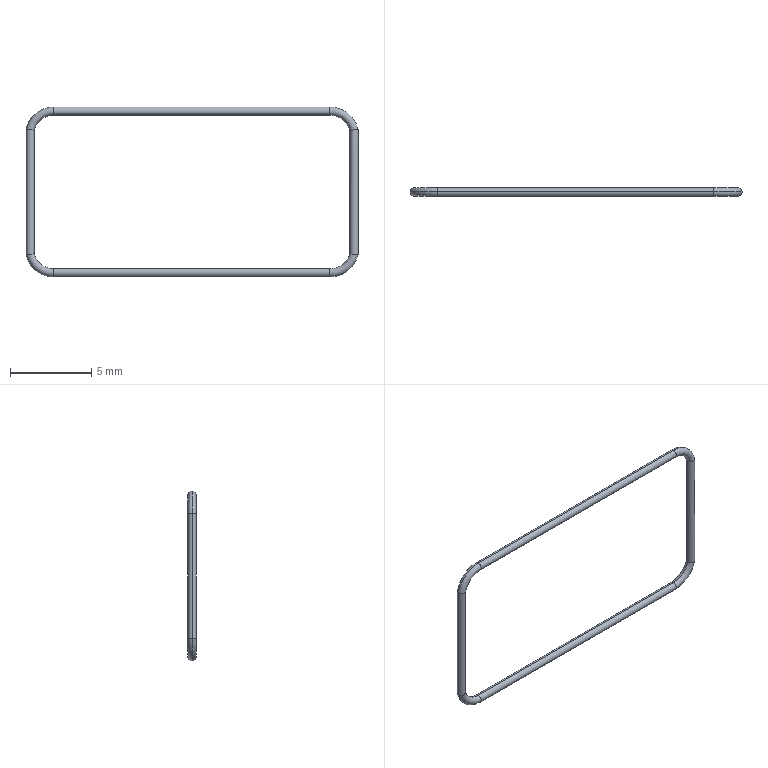Part | STEP file | XINAQUAN11_1_1_1 | 1 solid | 18 faces | box 20.47 x 0.5 x 10.48 mm | volume 11.282 mm3 | torus 8 | cylinder 8 | plane 2 | commonest cylinder face diameters 0.5 x8
STEP:
#1=CARTESIAN_POINT('',(0.,0.,0.));
#2=DIRECTION('',(0.,0.,1.));
#3=DIRECTION('',(1.,0.,0.));
#4=AXIS2_PLACEMENT_3D('',#1,#2,#3);
#5=CARTESIAN_POINT('',(8.51,0.,5.24));
#6=VERTEX_POINT('',#5);
#7=CARTESIAN_POINT('',(8.51,0.,4.74));
#8=VERTEX_POINT('',#7);
#9=CARTESIAN_POINT('',(8.51,0.,4.99));
#10=DIRECTION('',(-1.,0.,0.));
#11=DIRECTION('',(0.,0.,1.));
#12=AXIS2_PLACEMENT_3D('',#9,#10,#11);
#13=CIRCLE('',#12,0.25);
#14=EDGE_CURVE('',#6,#8,#13,.T.);
#15=ORIENTED_EDGE('',*,*,#14,.T.);
#16=CARTESIAN_POINT('',(9.758,0.,3.775));
#17=VERTEX_POINT('',#16);
#18=CARTESIAN_POINT('',(8.51,0.,3.45));
#19=DIRECTION('',(0.,1.,0.));
#20=DIRECTION('',(0.,0.,1.));
#21=AXIS2_PLACEMENT_3D('',#18,#19,#20);
#22=CIRCLE('',#21,1.29);
#23=EDGE_CURVE('',#8,#17,#22,.T.);
#24=ORIENTED_EDGE('',*,*,#23,.T.);
#25=CARTESIAN_POINT('',(10.242,0.,3.901));
#26=VERTEX_POINT('',#25);
#27=CARTESIAN_POINT('',(10.,0.,3.838));
#28=DIRECTION('',(-0.2522,0.,0.9677));
#29=DIRECTION('',(0.9677,0.,0.2522));
#30=AXIS2_PLACEMENT_3D('',#27,#28,#29);
#31=CIRCLE('',#30,0.25);
#32=EDGE_CURVE('',#26,#17,#31,.T.);
#33=ORIENTED_EDGE('',*,*,#32,.F.);
#34=CARTESIAN_POINT('',(8.51,0.,3.45));
#35=DIRECTION('',(0.,1.,0.));
#36=DIRECTION('',(0.,0.,1.));
#37=AXIS2_PLACEMENT_3D('',#34,#35,#36);
#38=CIRCLE('',#37,1.79);
#39=EDGE_CURVE('',#6,#26,#38,.T.);
#40=ORIENTED_EDGE('',*,*,#39,.F.);
#41=EDGE_LOOP('',(#15,#24,#33,#40));
#42=FACE_OUTER_BOUND('',#41,.F.);
#43=CARTESIAN_POINT('',(8.51,0.,3.45));
#44=DIRECTION('',(0.,1.,0.));
#45=DIRECTION('',(0.,0.,-1.));
#46=AXIS2_PLACEMENT_3D('',#43,#44,#45);
#47=TOROIDAL_SURFACE('',#46,1.54,0.25);
#48=ADVANCED_FACE('',(#42),#47,.T.);
#49=CARTESIAN_POINT('',(-8.51,0.,4.74));
#50=VERTEX_POINT('',#49);
#51=CARTESIAN_POINT('',(-8.51,0.,5.24));
#52=VERTEX_POINT('',#51);
#53=CARTESIAN_POINT('',(-8.51,0.,4.99));
#54=DIRECTION('',(1.,0.,0.));
#55=DIRECTION('',(0.,0.,-1.));
#56=AXIS2_PLACEMENT_3D('',#53,#54,#55);
#57=CIRCLE('',#56,0.25);
#58=EDGE_CURVE('',#50,#52,#57,.T.);
#59=ORIENTED_EDGE('',*,*,#58,.F.);
#60=CARTESIAN_POINT('',(-8.51,0.,4.74));
#61=DIRECTION('',(1.,0.,0.));
#62=VECTOR('',#61,17.02);
#63=LINE('',#60,#62);
#64=EDGE_CURVE('',#50,#8,#63,.T.);
#65=ORIENTED_EDGE('',*,*,#64,.T.);
#66=ORIENTED_EDGE('',*,*,#14,.F.);
#67=CARTESIAN_POINT('',(-8.51,0.,5.24));
#68=DIRECTION('',(1.,0.,0.));
#69=VECTOR('',#68,17.02);
#70=LINE('',#67,#69);
#71=EDGE_CURVE('',#52,#6,#70,.T.);
#72=ORIENTED_EDGE('',*,*,#71,.F.);
#73=EDGE_LOOP('',(#59,#65,#66,#72));
#74=FACE_OUTER_BOUND('',#73,.F.);
#75=CARTESIAN_POINT('',(-8.51,0.,4.99));
#76=DIRECTION('',(1.,0.,0.));
#77=DIRECTION('',(0.,0.,1.));
#78=AXIS2_PLACEMENT_3D('',#75,#76,#77);
#79=CYLINDRICAL_SURFACE('',#78,0.25);
#80=ADVANCED_FACE('',(#74),#79,.T.);
#81=CARTESIAN_POINT('',(-9.72,0.,3.805));
#82=VERTEX_POINT('',#81);
#83=CARTESIAN_POINT('',(-9.97,0.25,3.835));
#84=VERTEX_POINT('',#83);
#85=CARTESIAN_POINT('',(-9.72,0.02605,3.805));
#86=CARTESIAN_POINT('',(-9.728,0.0782,3.806));
#87=CARTESIAN_POINT('',(-9.764,0.1492,3.81));
#88=CARTESIAN_POINT('',(-9.82,0.2053,3.817));
#89=CARTESIAN_POINT('',(-9.891,0.2416,3.826));
#90=CARTESIAN_POINT('',(-9.943,0.25,3.832));
#91=B_SPLINE_CURVE_WITH_KNOTS('',3,(#81,#85,#86,#87,#88,#89,#90,#83),.UNSPECIFIED.,.F.,.F.,(4,1,1,1,1,4),(0.,0.2,0.4,0.6,0.8,1.),.UNSPECIFIED.);
#92=EDGE_CURVE('',#82,#84,#91,.T.);
#93=ORIENTED_EDGE('',*,*,#92,.F.);
#94=CARTESIAN_POINT('',(-8.51,0.,3.49));
#95=DIRECTION('',(0.,1.,0.));
#96=DIRECTION('',(-0.9678,0.,0.2516));
#97=AXIS2_PLACEMENT_3D('',#94,#95,#96);
#98=CIRCLE('',#97,1.25);
#99=EDGE_CURVE('',#82,#50,#98,.T.);
#100=ORIENTED_EDGE('',*,*,#99,.T.);
#101=ORIENTED_EDGE('',*,*,#58,.T.);
#102=CARTESIAN_POINT('',(-10.213,0.,3.893));
#103=VERTEX_POINT('',#102);
#104=CARTESIAN_POINT('',(-8.51,0.,3.49));
#105=DIRECTION('',(0.,1.,0.));
#106=DIRECTION('',(-0.9732,0.,0.23));
#107=AXIS2_PLACEMENT_3D('',#104,#105,#106);
#108=CIRCLE('',#107,1.75);
#109=EDGE_CURVE('',#103,#52,#108,.T.);
#110=ORIENTED_EDGE('',*,*,#109,.F.);
#111=CARTESIAN_POINT('',(-10.22,0.,3.863));
#112=VERTEX_POINT('',#111);
#113=CARTESIAN_POINT('',(-8.51,0.,3.49));
#114=DIRECTION('',(0.,1.,0.));
#115=DIRECTION('',(-0.977,0.,0.2131));
#116=AXIS2_PLACEMENT_3D('',#113,#114,#115);
#117=CIRCLE('',#116,1.75);
#118=EDGE_CURVE('',#112,#103,#117,.T.);
#119=ORIENTED_EDGE('',*,*,#118,.F.);
#120=CARTESIAN_POINT('',(-9.97,0.25,3.835));
#121=CARTESIAN_POINT('',(-9.996,0.25,3.838));
#122=CARTESIAN_POINT('',(-10.049,0.2416,3.844));
#123=CARTESIAN_POINT('',(-10.119,0.2055,3.852));
#124=CARTESIAN_POINT('',(-10.176,0.1491,3.858));
#125=CARTESIAN_POINT('',(-10.212,0.07816,3.862));
#126=CARTESIAN_POINT('',(-10.22,0.02602,3.863));
#127=CARTESIAN_POINT('',(-10.22,0.,3.863));
#128=B_SPLINE_CURVE_WITH_KNOTS('',3,(#120,#121,#122,#123,#124,#125,#126,#127),.UNSPECIFIED.,.F.,.F.,(4,1,1,1,1,4),(0.,0.2,0.4,0.6,0.8,1.),.UNSPECIFIED.);
#129=EDGE_CURVE('',#84,#112,#128,.T.);
#130=ORIENTED_EDGE('',*,*,#129,.F.);
#131=EDGE_LOOP('',(#93,#100,#101,#110,#119,#130));
#132=FACE_OUTER_BOUND('',#131,.F.);
#133=CARTESIAN_POINT('',(-8.51,0.,3.49));
#134=DIRECTION('',(0.,1.,0.));
#135=DIRECTION('',(0.9732,0.,-0.23));
#136=AXIS2_PLACEMENT_3D('',#133,#134,#135);
#137=TOROIDAL_SURFACE('',#136,1.5,0.25);
#138=ADVANCED_FACE('',(#132),#137,.T.);
#139=CARTESIAN_POINT('',(-9.72,0.,-3.805));
#140=VERTEX_POINT('',#139);
#141=CARTESIAN_POINT('',(-9.97,0.25,-3.835));
#142=VERTEX_POINT('',#141);
#143=CARTESIAN_POINT('',(-9.72,0.02606,-3.805));
#144=CARTESIAN_POINT('',(-9.728,0.07824,-3.806));
#145=CARTESIAN_POINT('',(-9.764,0.1492,-3.81));
#146=CARTESIAN_POINT('',(-9.82,0.2054,-3.817));
#147=CARTESIAN_POINT('',(-9.891,0.2416,-3.826));
#148=CARTESIAN_POINT('',(-9.943,0.25,-3.832));
#149=B_SPLINE_CURVE_WITH_KNOTS('',3,(#139,#143,#144,#145,#146,#147,#148,#141),.UNSPECIFIED.,.F.,.F.,(4,1,1,1,1,4),(0.,0.2,0.4,0.6,0.8,1.),.UNSPECIFIED.);
#150=EDGE_CURVE('',#140,#142,#149,.T.);
#151=ORIENTED_EDGE('',*,*,#150,.F.);
#152=CARTESIAN_POINT('',(-9.72,0.,-3.805));
#153=DIRECTION('',(0.,0.,1.));
#154=VECTOR('',#153,7.609);
#155=LINE('',#152,#154);
#156=EDGE_CURVE('',#140,#82,#155,.T.);
#157=ORIENTED_EDGE('',*,*,#156,.T.);
#158=ORIENTED_EDGE('',*,*,#92,.T.);
#159=ORIENTED_EDGE('',*,*,#129,.T.);
#160=CARTESIAN_POINT('',(-10.22,0.,-3.863));
#161=VERTEX_POINT('',#160);
#162=CARTESIAN_POINT('',(-10.22,0.,-3.863));
#163=DIRECTION('',(0.,0.,1.));
#164=VECTOR('',#163,7.726);
#165=LINE('',#162,#164);
#166=EDGE_CURVE('',#161,#112,#165,.T.);
#167=ORIENTED_EDGE('',*,*,#166,.F.);
#168=CARTESIAN_POINT('',(-9.97,0.25,-3.835));
#169=CARTESIAN_POINT('',(-9.996,0.25,-3.838));
#170=CARTESIAN_POINT('',(-10.049,0.2416,-3.844));
#171=CARTESIAN_POINT('',(-10.119,0.2055,-3.852));
#172=CARTESIAN_POINT('',(-10.176,0.1491,-3.858));
#173=CARTESIAN_POINT('',(-10.212,0.07808,-3.862));
#174=CARTESIAN_POINT('',(-10.22,0.02599,-3.863));
#175=CARTESIAN_POINT('',(-10.22,0.,-3.863));
#176=B_SPLINE_CURVE_WITH_KNOTS('',3,(#168,#169,#170,#171,#172,#173,#174,#175),.UNSPECIFIED.,.F.,.F.,(4,1,1,1,1,4),(0.,0.2,0.4,0.6,0.8,1.),.UNSPECIFIED.);
#177=EDGE_CURVE('',#142,#161,#176,.T.);
#178=ORIENTED_EDGE('',*,*,#177,.F.);
#179=EDGE_LOOP('',(#151,#157,#158,#159,#167,#178));
#180=FACE_OUTER_BOUND('',#179,.F.);
#181=CARTESIAN_POINT('',(-9.97,0.,-3.835));
#182=DIRECTION('',(0.,0.,1.));
#183=DIRECTION('',(-1.,0.,0.));
#184=AXIS2_PLACEMENT_3D('',#181,#182,#183);
#185=CYLINDRICAL_SURFACE('',#184,0.25);
#186=ADVANCED_FACE('',(#180),#185,.T.);
#187=CARTESIAN_POINT('',(-8.51,0.,-5.24));
#188=VERTEX_POINT('',#187);
#189=CARTESIAN_POINT('',(-8.51,0.,-4.74));
#190=VERTEX_POINT('',#189);
#191=CARTESIAN_POINT('',(-8.51,0.,-4.99));
#192=DIRECTION('',(1.,0.,0.));
#193=DIRECTION('',(0.,0.,-1.));
#194=AXIS2_PLACEMENT_3D('',#191,#192,#193);
#195=CIRCLE('',#194,0.25);
#196=EDGE_CURVE('',#188,#190,#195,.T.);
#197=ORIENTED_EDGE('',*,*,#196,.T.);
#198=CARTESIAN_POINT('',(-8.51,0.,-3.49));
#199=DIRECTION('',(0.,1.,0.));
#200=DIRECTION('',(0.,0.,-1.));
#201=AXIS2_PLACEMENT_3D('',#198,#199,#200);
#202=CIRCLE('',#201,1.25);
#203=EDGE_CURVE('',#190,#140,#202,.T.);
#204=ORIENTED_EDGE('',*,*,#203,.T.);
#205=ORIENTED_EDGE('',*,*,#150,.T.);
#206=ORIENTED_EDGE('',*,*,#177,.T.);
#207=CARTESIAN_POINT('',(-8.51,0.,-3.49));
#208=DIRECTION('',(0.,1.,0.));
#209=DIRECTION('',(0.,0.,-1.));
#210=AXIS2_PLACEMENT_3D('',#207,#208,#209);
#211=CIRCLE('',#210,1.75);
#212=EDGE_CURVE('',#188,#161,#211,.T.);
#213=ORIENTED_EDGE('',*,*,#212,.F.);
#214=EDGE_LOOP('',(#197,#204,#205,#206,#213));
#215=FACE_OUTER_BOUND('',#214,.F.);
#216=CARTESIAN_POINT('',(-8.51,0.,-3.49));
#217=DIRECTION('',(0.,1.,0.));
#218=DIRECTION('',(0.,0.,1.));
#219=AXIS2_PLACEMENT_3D('',#216,#217,#218);
#220=TOROIDAL_SURFACE('',#219,1.5,0.25);
#221=ADVANCED_FACE('',(#215),#220,.T.);
#222=CARTESIAN_POINT('',(8.51,0.,-4.74));
#223=VERTEX_POINT('',#222);
#224=CARTESIAN_POINT('',(8.51,0.,-5.24));
#225=VERTEX_POINT('',#224);
#226=CARTESIAN_POINT('',(8.51,0.,-4.99));
#227=DIRECTION('',(-1.,0.,0.));
#228=DIRECTION('',(0.,0.,1.));
#229=AXIS2_PLACEMENT_3D('',#226,#227,#228);
#230=CIRCLE('',#229,0.25);
#231=EDGE_CURVE('',#223,#225,#230,.T.);
#232=ORIENTED_EDGE('',*,*,#231,.F.);
#233=CARTESIAN_POINT('',(8.51,0.,-4.74));
#234=DIRECTION('',(-1.,0.,0.));
#235=VECTOR('',#234,17.02);
#236=LINE('',#233,#235);
#237=EDGE_CURVE('',#223,#190,#236,.T.);
#238=ORIENTED_EDGE('',*,*,#237,.T.);
#239=ORIENTED_EDGE('',*,*,#196,.F.);
#240=CARTESIAN_POINT('',(8.51,0.,-5.24));
#241=DIRECTION('',(-1.,0.,0.));
#242=VECTOR('',#241,17.02);
#243=LINE('',#240,#242);
#244=EDGE_CURVE('',#225,#188,#243,.T.);
#245=ORIENTED_EDGE('',*,*,#244,.F.);
#246=EDGE_LOOP('',(#232,#238,#239,#245));
#247=FACE_OUTER_BOUND('',#246,.F.);
#248=CARTESIAN_POINT('',(8.51,0.,-4.99));
#249=DIRECTION('',(-1.,0.,0.));
#250=DIRECTION('',(0.,0.,-1.));
#251=AXIS2_PLACEMENT_3D('',#248,#249,#250);
#252=CYLINDRICAL_SURFACE('',#251,0.25);
#253=ADVANCED_FACE('',(#247),#252,.T.);
#254=CARTESIAN_POINT('',(9.75,0.,-3.805));
#255=VERTEX_POINT('',#254);
#256=CARTESIAN_POINT('',(10.,0.25,-3.838));
#257=VERTEX_POINT('',#256);
#258=CARTESIAN_POINT('',(9.75,0.02603,-3.805));
#259=CARTESIAN_POINT('',(9.758,0.07815,-3.806));
#260=CARTESIAN_POINT('',(9.794,0.1491,-3.811));
#261=CARTESIAN_POINT('',(9.85,0.2053,-3.819));
#262=CARTESIAN_POINT('',(9.921,0.2415,-3.828));
#263=CARTESIAN_POINT('',(9.974,0.25,-3.835));
#264=B_SPLINE_CURVE_WITH_KNOTS('',3,(#254,#258,#259,#260,#261,#262,#263,#256),.UNSPECIFIED.,.F.,.F.,(4,1,1,1,1,4),(0.,0.2,0.4,0.6,0.8,1.),.UNSPECIFIED.);
#265=EDGE_CURVE('',#255,#257,#264,.T.);
#266=ORIENTED_EDGE('',*,*,#265,.F.);
#267=CARTESIAN_POINT('',(8.51,0.,-3.45));
#268=DIRECTION('',(0.,1.,0.));
#269=DIRECTION('',(0.9614,0.,-0.2751));
#270=AXIS2_PLACEMENT_3D('',#267,#268,#269);
#271=CIRCLE('',#270,1.29);
#272=EDGE_CURVE('',#255,#223,#271,.T.);
#273=ORIENTED_EDGE('',*,*,#272,.T.);
#274=ORIENTED_EDGE('',*,*,#231,.T.);
#275=CARTESIAN_POINT('',(10.242,0.,-3.901));
#276=VERTEX_POINT('',#275);
#277=CARTESIAN_POINT('',(8.51,0.,-3.45));
#278=DIRECTION('',(0.,1.,0.));
#279=DIRECTION('',(0.9677,0.,-0.2522));
#280=AXIS2_PLACEMENT_3D('',#277,#278,#279);
#281=CIRCLE('',#280,1.79);
#282=EDGE_CURVE('',#276,#225,#281,.T.);
#283=ORIENTED_EDGE('',*,*,#282,.F.);
#284=CARTESIAN_POINT('',(10.25,0.,-3.869));
#285=VERTEX_POINT('',#284);
#286=CARTESIAN_POINT('',(8.51,0.,-3.45));
#287=DIRECTION('',(0.,1.,0.));
#288=DIRECTION('',(0.9722,0.,-0.2342));
#289=AXIS2_PLACEMENT_3D('',#286,#287,#288);
#290=CIRCLE('',#289,1.79);
#291=EDGE_CURVE('',#285,#276,#290,.T.);
#292=ORIENTED_EDGE('',*,*,#291,.F.);
#293=CARTESIAN_POINT('',(10.,0.25,-3.838));
#294=CARTESIAN_POINT('',(10.027,0.25,-3.842));
#295=CARTESIAN_POINT('',(10.079,0.2416,-3.848));
#296=CARTESIAN_POINT('',(10.15,0.2055,-3.857));
#297=CARTESIAN_POINT('',(10.206,0.1491,-3.864));
#298=CARTESIAN_POINT('',(10.242,0.07799,-3.868));
#299=CARTESIAN_POINT('',(10.25,0.02595,-3.869));
#300=CARTESIAN_POINT('',(10.25,0.,-3.869));
#301=B_SPLINE_CURVE_WITH_KNOTS('',3,(#293,#294,#295,#296,#297,#298,#299,#300),.UNSPECIFIED.,.F.,.F.,(4,1,1,1,1,4),(0.,0.2,0.4,0.6,0.8,1.),.UNSPECIFIED.);
#302=EDGE_CURVE('',#257,#285,#301,.T.);
#303=ORIENTED_EDGE('',*,*,#302,.F.);
#304=EDGE_LOOP('',(#266,#273,#274,#283,#292,#303));
#305=FACE_OUTER_BOUND('',#304,.F.);
#306=CARTESIAN_POINT('',(8.51,0.,-3.45));
#307=DIRECTION('',(0.,1.,0.));
#308=DIRECTION('',(-0.9677,0.,0.2522));
#309=AXIS2_PLACEMENT_3D('',#306,#307,#308);
#310=TOROIDAL_SURFACE('',#309,1.54,0.25);
#311=ADVANCED_FACE('',(#305),#310,.T.);
#312=CARTESIAN_POINT('',(9.75,0.,3.842));
#313=VERTEX_POINT('',#312);
#314=CARTESIAN_POINT('',(10.25,0.,3.842));
#315=VERTEX_POINT('',#314);
#316=CARTESIAN_POINT('',(10.,0.,3.842));
#317=DIRECTION('',(0.,0.,-1.));
#318=DIRECTION('',(-1.,0.,0.));
#319=AXIS2_PLACEMENT_3D('',#316,#317,#318);
#320=CIRCLE('',#319,0.25);
#321=EDGE_CURVE('',#313,#315,#320,.T.);
#322=ORIENTED_EDGE('',*,*,#321,.F.);
#323=CARTESIAN_POINT('',(9.75,0.,3.842));
#324=DIRECTION('',(0.,0.,-1.));
#325=VECTOR('',#324,7.647);
#326=LINE('',#323,#325);
#327=EDGE_CURVE('',#313,#255,#326,.T.);
#328=ORIENTED_EDGE('',*,*,#327,.T.);
#329=ORIENTED_EDGE('',*,*,#265,.T.);
#330=ORIENTED_EDGE('',*,*,#302,.T.);
#331=CARTESIAN_POINT('',(10.25,0.,3.842));
#332=DIRECTION('',(0.,0.,-1.));
#333=VECTOR('',#332,7.711);
#334=LINE('',#331,#333);
#335=EDGE_CURVE('',#315,#285,#334,.T.);
#336=ORIENTED_EDGE('',*,*,#335,.F.);
#337=EDGE_LOOP('',(#322,#328,#329,#330,#336));
#338=FACE_OUTER_BOUND('',#337,.F.);
#339=CARTESIAN_POINT('',(10.,0.,3.842));
#340=DIRECTION('',(0.,0.,-1.));
#341=DIRECTION('',(1.,0.,0.));
#342=AXIS2_PLACEMENT_3D('',#339,#340,#341);
#343=CYLINDRICAL_SURFACE('',#342,0.25);
#344=ADVANCED_FACE('',(#338),#343,.T.);
#345=CARTESIAN_POINT('',(10.,0.,3.842));
#346=DIRECTION('',(0.,0.,-1.));
#347=DIRECTION('',(1.,0.,0.));
#348=AXIS2_PLACEMENT_3D('',#345,#346,#347);
#349=CIRCLE('',#348,0.25);
#350=EDGE_CURVE('',#315,#313,#349,.T.);
#351=ORIENTED_EDGE('',*,*,#350,.T.);
#352=ORIENTED_EDGE('',*,*,#321,.T.);
#353=EDGE_LOOP('',(#351,#352));
#354=FACE_OUTER_BOUND('',#353,.F.);
#355=CARTESIAN_POINT('',(10.,0.,3.842));
#356=DIRECTION('',(0.,0.,-1.));
#357=DIRECTION('',(1.,0.,0.));
#358=AXIS2_PLACEMENT_3D('',#355,#356,#357);
#359=PLANE('',#358);
#360=ADVANCED_FACE('',(#354),#359,.F.);
#361=ORIENTED_EDGE('',*,*,#350,.F.);
#362=ORIENTED_EDGE('',*,*,#335,.T.);
#363=CARTESIAN_POINT('',(10.,-0.25,-3.838));
#364=VERTEX_POINT('',#363);
#365=CARTESIAN_POINT('',(10.25,0.,-3.869));
#366=CARTESIAN_POINT('',(10.25,-0.02609,-3.869));
#367=CARTESIAN_POINT('',(10.242,-0.0783,-3.868));
#368=CARTESIAN_POINT('',(10.206,-0.1492,-3.864));
#369=CARTESIAN_POINT('',(10.15,-0.2054,-3.857));
#370=CARTESIAN_POINT('',(10.079,-0.2415,-3.848));
#371=CARTESIAN_POINT('',(10.027,-0.25,-3.842));
#372=B_SPLINE_CURVE_WITH_KNOTS('',3,(#365,#366,#367,#368,#369,#370,#371,#363),.UNSPECIFIED.,.F.,.F.,(4,1,1,1,1,4),(0.,0.2,0.4,0.6,0.8,1.),.UNSPECIFIED.);
#373=EDGE_CURVE('',#285,#364,#372,.T.);
#374=ORIENTED_EDGE('',*,*,#373,.T.);
#375=CARTESIAN_POINT('',(10.,-0.25,-3.838));
#376=CARTESIAN_POINT('',(9.974,-0.25,-3.835));
#377=CARTESIAN_POINT('',(9.921,-0.2416,-3.828));
#378=CARTESIAN_POINT('',(9.851,-0.2054,-3.819));
#379=CARTESIAN_POINT('',(9.794,-0.1491,-3.811));
#380=CARTESIAN_POINT('',(9.758,-0.07787,-3.806));
#381=CARTESIAN_POINT('',(9.75,-0.02589,-3.805));
#382=CARTESIAN_POINT('',(9.75,0.,-3.805));
#383=B_SPLINE_CURVE_WITH_KNOTS('',3,(#375,#376,#377,#378,#379,#380,#381,#382),.UNSPECIFIED.,.F.,.F.,(4,1,1,1,1,4),(0.,0.2,0.4,0.6,0.8,1.),.UNSPECIFIED.);
#384=EDGE_CURVE('',#364,#255,#383,.T.);
#385=ORIENTED_EDGE('',*,*,#384,.T.);
#386=ORIENTED_EDGE('',*,*,#327,.F.);
#387=EDGE_LOOP('',(#361,#362,#374,#385,#386));
#388=FACE_OUTER_BOUND('',#387,.F.);
#389=CARTESIAN_POINT('',(10.,0.,3.842));
#390=DIRECTION('',(0.,0.,-1.));
#391=DIRECTION('',(1.,0.,0.));
#392=AXIS2_PLACEMENT_3D('',#389,#390,#391);
#393=CYLINDRICAL_SURFACE('',#392,0.25);
#394=ADVANCED_FACE('',(#388),#393,.T.);
#395=ORIENTED_EDGE('',*,*,#373,.F.);
#396=ORIENTED_EDGE('',*,*,#291,.T.);
#397=ORIENTED_EDGE('',*,*,#282,.T.);
#398=CARTESIAN_POINT('',(8.51,0.,-4.99));
#399=DIRECTION('',(-1.,0.,0.));
#400=DIRECTION('',(0.,0.,-1.));
#401=AXIS2_PLACEMENT_3D('',#398,#399,#400);
#402=CIRCLE('',#401,0.25);
#403=EDGE_CURVE('',#225,#223,#402,.T.);
#404=ORIENTED_EDGE('',*,*,#403,.T.);
#405=ORIENTED_EDGE('',*,*,#272,.F.);
#406=ORIENTED_EDGE('',*,*,#384,.F.);
#407=EDGE_LOOP('',(#395,#396,#397,#404,#405,#406));
#408=FACE_OUTER_BOUND('',#407,.F.);
#409=CARTESIAN_POINT('',(8.51,0.,-3.45));
#410=DIRECTION('',(0.,1.,0.));
#411=DIRECTION('',(-0.9677,0.,0.2522));
#412=AXIS2_PLACEMENT_3D('',#409,#410,#411);
#413=TOROIDAL_SURFACE('',#412,1.54,0.25);
#414=ADVANCED_FACE('',(#408),#413,.T.);
#415=ORIENTED_EDGE('',*,*,#403,.F.);
#416=ORIENTED_EDGE('',*,*,#244,.T.);
#417=CARTESIAN_POINT('',(-8.51,0.,-4.99));
#418=DIRECTION('',(1.,0.,0.));
#419=DIRECTION('',(0.,0.,1.));
#420=AXIS2_PLACEMENT_3D('',#417,#418,#419);
#421=CIRCLE('',#420,0.25);
#422=EDGE_CURVE('',#190,#188,#421,.T.);
#423=ORIENTED_EDGE('',*,*,#422,.F.);
#424=ORIENTED_EDGE('',*,*,#237,.F.);
#425=EDGE_LOOP('',(#415,#416,#423,#424));
#426=FACE_OUTER_BOUND('',#425,.F.);
#427=CARTESIAN_POINT('',(8.51,0.,-4.99));
#428=DIRECTION('',(-1.,0.,0.));
#429=DIRECTION('',(0.,0.,-1.));
#430=AXIS2_PLACEMENT_3D('',#427,#428,#429);
#431=CYLINDRICAL_SURFACE('',#430,0.25);
#432=ADVANCED_FACE('',(#426),#431,.T.);
#433=ORIENTED_EDGE('',*,*,#422,.T.);
#434=ORIENTED_EDGE('',*,*,#212,.T.);
#435=CARTESIAN_POINT('',(-9.97,-0.25,-3.835));
#436=VERTEX_POINT('',#435);
#437=CARTESIAN_POINT('',(-10.22,0.,-3.863));
#438=CARTESIAN_POINT('',(-10.22,-0.02609,-3.863));
#439=CARTESIAN_POINT('',(-10.212,-0.07831,-3.862));
#440=CARTESIAN_POINT('',(-10.175,-0.1493,-3.858));
#441=CARTESIAN_POINT('',(-10.119,-0.2054,-3.852));
#442=CARTESIAN_POINT('',(-10.049,-0.2416,-3.844));
#443=CARTESIAN_POINT('',(-9.996,-0.25,-3.838));
#444=B_SPLINE_CURVE_WITH_KNOTS('',3,(#437,#438,#439,#440,#441,#442,#443,#435),.UNSPECIFIED.,.F.,.F.,(4,1,1,1,1,4),(0.,0.2,0.4,0.6,0.8,1.),.UNSPECIFIED.);
#445=EDGE_CURVE('',#161,#436,#444,.T.);
#446=ORIENTED_EDGE('',*,*,#445,.T.);
#447=CARTESIAN_POINT('',(-9.97,-0.25,-3.835));
#448=CARTESIAN_POINT('',(-9.943,-0.25,-3.832));
#449=CARTESIAN_POINT('',(-9.891,-0.2416,-3.826));
#450=CARTESIAN_POINT('',(-9.82,-0.2055,-3.817));
#451=CARTESIAN_POINT('',(-9.764,-0.1491,-3.81));
#452=CARTESIAN_POINT('',(-9.728,-0.07808,-3.806));
#453=CARTESIAN_POINT('',(-9.72,-0.02598,-3.805));
#454=CARTESIAN_POINT('',(-9.72,0.,-3.805));
#455=B_SPLINE_CURVE_WITH_KNOTS('',3,(#447,#448,#449,#450,#451,#452,#453,#454),.UNSPECIFIED.,.F.,.F.,(4,1,1,1,1,4),(0.,0.2,0.4,0.6,0.8,1.),.UNSPECIFIED.);
#456=EDGE_CURVE('',#436,#140,#455,.T.);
#457=ORIENTED_EDGE('',*,*,#456,.T.);
#458=ORIENTED_EDGE('',*,*,#203,.F.);
#459=EDGE_LOOP('',(#433,#434,#446,#457,#458));
#460=FACE_OUTER_BOUND('',#459,.F.);
#461=CARTESIAN_POINT('',(-8.51,0.,-3.49));
#462=DIRECTION('',(0.,1.,0.));
#463=DIRECTION('',(0.,0.,1.));
#464=AXIS2_PLACEMENT_3D('',#461,#462,#463);
#465=TOROIDAL_SURFACE('',#464,1.5,0.25);
#466=ADVANCED_FACE('',(#460),#465,.T.);
#467=ORIENTED_EDGE('',*,*,#445,.F.);
#468=ORIENTED_EDGE('',*,*,#166,.T.);
#469=CARTESIAN_POINT('',(-9.97,-0.25,3.835));
#470=VERTEX_POINT('',#469);
#471=CARTESIAN_POINT('',(-10.22,0.,3.863));
#472=CARTESIAN_POINT('',(-10.22,-0.0261,3.863));
#473=CARTESIAN_POINT('',(-10.212,-0.07833,3.862));
#474=CARTESIAN_POINT('',(-10.175,-0.1493,3.858));
#475=CARTESIAN_POINT('',(-10.119,-0.2054,3.852));
#476=CARTESIAN_POINT('',(-10.049,-0.2416,3.844));
#477=CARTESIAN_POINT('',(-9.996,-0.25,3.838));
#478=B_SPLINE_CURVE_WITH_KNOTS('',3,(#471,#472,#473,#474,#475,#476,#477,#469),.UNSPECIFIED.,.F.,.F.,(4,1,1,1,1,4),(0.,0.2,0.4,0.6,0.8,1.),.UNSPECIFIED.);
#479=EDGE_CURVE('',#112,#470,#478,.T.);
#480=ORIENTED_EDGE('',*,*,#479,.T.);
#481=CARTESIAN_POINT('',(-9.97,-0.25,3.835));
#482=CARTESIAN_POINT('',(-9.943,-0.25,3.832));
#483=CARTESIAN_POINT('',(-9.891,-0.2416,3.826));
#484=CARTESIAN_POINT('',(-9.82,-0.2055,3.817));
#485=CARTESIAN_POINT('',(-9.764,-0.149,3.81));
#486=CARTESIAN_POINT('',(-9.728,-0.07807,3.806));
#487=CARTESIAN_POINT('',(-9.72,-0.02598,3.805));
#488=CARTESIAN_POINT('',(-9.72,0.,3.805));
#489=B_SPLINE_CURVE_WITH_KNOTS('',3,(#481,#482,#483,#484,#485,#486,#487,#488),.UNSPECIFIED.,.F.,.F.,(4,1,1,1,1,4),(0.,0.2,0.4,0.6,0.8,1.),.UNSPECIFIED.);
#490=EDGE_CURVE('',#470,#82,#489,.T.);
#491=ORIENTED_EDGE('',*,*,#490,.T.);
#492=ORIENTED_EDGE('',*,*,#156,.F.);
#493=ORIENTED_EDGE('',*,*,#456,.F.);
#494=EDGE_LOOP('',(#467,#468,#480,#491,#492,#493));
#495=FACE_OUTER_BOUND('',#494,.F.);
#496=CARTESIAN_POINT('',(-9.97,0.,-3.835));
#497=DIRECTION('',(0.,0.,1.));
#498=DIRECTION('',(-1.,0.,0.));
#499=AXIS2_PLACEMENT_3D('',#496,#497,#498);
#500=CYLINDRICAL_SURFACE('',#499,0.25);
#501=ADVANCED_FACE('',(#495),#500,.T.);
#502=ORIENTED_EDGE('',*,*,#479,.F.);
#503=ORIENTED_EDGE('',*,*,#118,.T.);
#504=ORIENTED_EDGE('',*,*,#109,.T.);
#505=CARTESIAN_POINT('',(-8.51,0.,4.99));
#506=DIRECTION('',(1.,0.,0.));
#507=DIRECTION('',(0.,0.,1.));
#508=AXIS2_PLACEMENT_3D('',#505,#506,#507);
#509=CIRCLE('',#508,0.25);
#510=EDGE_CURVE('',#52,#50,#509,.T.);
#511=ORIENTED_EDGE('',*,*,#510,.T.);
#512=ORIENTED_EDGE('',*,*,#99,.F.);
#513=ORIENTED_EDGE('',*,*,#490,.F.);
#514=EDGE_LOOP('',(#502,#503,#504,#511,#512,#513));
#515=FACE_OUTER_BOUND('',#514,.F.);
#516=CARTESIAN_POINT('',(-8.51,0.,3.49));
#517=DIRECTION('',(0.,1.,0.));
#518=DIRECTION('',(0.9732,0.,-0.23));
#519=AXIS2_PLACEMENT_3D('',#516,#517,#518);
#520=TOROIDAL_SURFACE('',#519,1.5,0.25);
#521=ADVANCED_FACE('',(#515),#520,.T.);
#522=ORIENTED_EDGE('',*,*,#510,.F.);
#523=ORIENTED_EDGE('',*,*,#71,.T.);
#524=CARTESIAN_POINT('',(8.51,0.,4.99));
#525=DIRECTION('',(-1.,0.,0.));
#526=DIRECTION('',(0.,0.,-1.));
#527=AXIS2_PLACEMENT_3D('',#524,#525,#526);
#528=CIRCLE('',#527,0.25);
#529=EDGE_CURVE('',#8,#6,#528,.T.);
#530=ORIENTED_EDGE('',*,*,#529,.F.);
#531=ORIENTED_EDGE('',*,*,#64,.F.);
#532=EDGE_LOOP('',(#522,#523,#530,#531));
#533=FACE_OUTER_BOUND('',#532,.F.);
#534=CARTESIAN_POINT('',(-8.51,0.,4.99));
#535=DIRECTION('',(1.,0.,0.));
#536=DIRECTION('',(0.,0.,1.));
#537=AXIS2_PLACEMENT_3D('',#534,#535,#536);
#538=CYLINDRICAL_SURFACE('',#537,0.25);
#539=ADVANCED_FACE('',(#533),#538,.T.);
#540=ORIENTED_EDGE('',*,*,#529,.T.);
#541=ORIENTED_EDGE('',*,*,#39,.T.);
#542=CARTESIAN_POINT('',(10.,0.,3.838));
#543=DIRECTION('',(-0.2522,0.,0.9677));
#544=DIRECTION('',(-0.9677,0.,-0.2522));
#545=AXIS2_PLACEMENT_3D('',#542,#543,#544);
#546=CIRCLE('',#545,0.25);
#547=EDGE_CURVE('',#17,#26,#546,.T.);
#548=ORIENTED_EDGE('',*,*,#547,.F.);
#549=ORIENTED_EDGE('',*,*,#23,.F.);
#550=EDGE_LOOP('',(#540,#541,#548,#549));
#551=FACE_OUTER_BOUND('',#550,.F.);
#552=CARTESIAN_POINT('',(8.51,0.,3.45));
#553=DIRECTION('',(0.,1.,0.));
#554=DIRECTION('',(0.,0.,-1.));
#555=AXIS2_PLACEMENT_3D('',#552,#553,#554);
#556=TOROIDAL_SURFACE('',#555,1.54,0.25);
#557=ADVANCED_FACE('',(#551),#556,.T.);
#558=ORIENTED_EDGE('',*,*,#547,.T.);
#559=ORIENTED_EDGE('',*,*,#32,.T.);
#560=EDGE_LOOP('',(#558,#559));
#561=FACE_OUTER_BOUND('',#560,.F.);
#562=CARTESIAN_POINT('',(8.51,-1.,3.45));
#563=DIRECTION('',(0.2522,0.,-0.9677));
#564=DIRECTION('',(-0.9677,0.,-0.2522));
#565=AXIS2_PLACEMENT_3D('',#562,#563,#564);
#566=PLANE('',#565);
#567=ADVANCED_FACE('',(#561),#566,.T.);
#568=CLOSED_SHELL('',(#48,#80,#138,#186,#221,#253,#311,#344,#360,#394,#414,#432,#466,#501,#521,#539,#557,#567));
#569=MANIFOLD_SOLID_BREP('',#568);
#570=(LENGTH_UNIT()NAMED_UNIT(*)SI_UNIT(.MILLI.,.METRE.));
#571=UNCERTAINTY_MEASURE_WITH_UNIT(LENGTH_MEASURE(0.0023),#570,'','');
#572=(NAMED_UNIT(*)PLANE_ANGLE_UNIT()SI_UNIT($,.RADIAN.));
#573=PLANE_ANGLE_MEASURE_WITH_UNIT(PLANE_ANGLE_MEASURE(0.01745),#572);
#574=(CONVERSION_BASED_UNIT('DEGREE',#573)NAMED_UNIT(*)PLANE_ANGLE_UNIT());
#575=(NAMED_UNIT(*)SI_UNIT($,.STERADIAN.)SOLID_ANGLE_UNIT());
#576=(GEOMETRIC_REPRESENTATION_CONTEXT(3)GLOBAL_UNCERTAINTY_ASSIGNED_CONTEXT((#571))GLOBAL_UNIT_ASSIGNED_CONTEXT((#570,#574,#575))REPRESENTATION_CONTEXT('',''));
#577=ADVANCED_BREP_SHAPE_REPRESENTATION('',(#4,#569),#576);